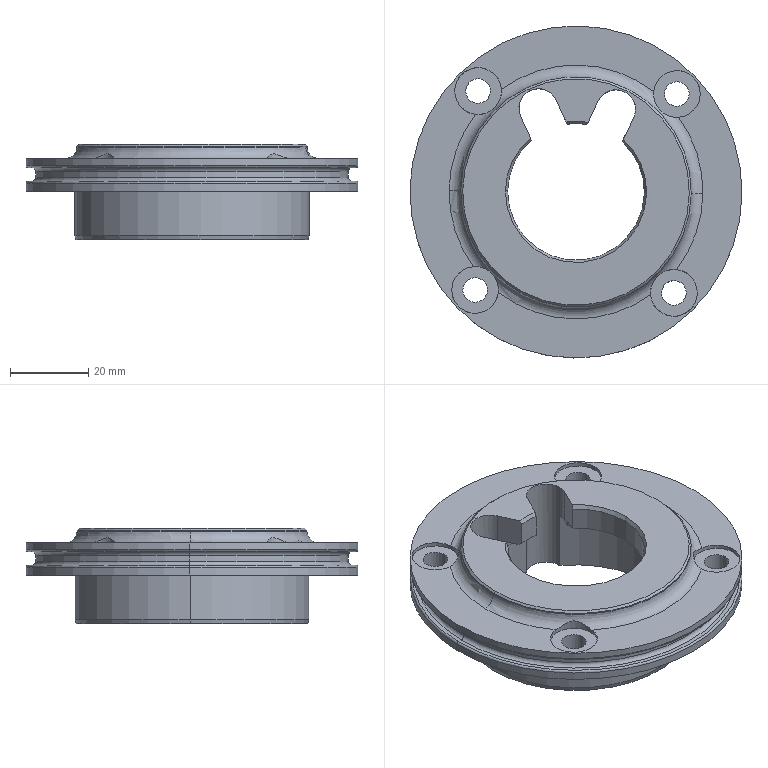Part | SolidWorks | features BaseBody 1 | 1 solid | 81 faces | box 85 x 85 x 24.5 mm | volume 44441 mm3 | cylinder 41 | plane 18 | cone 12 | torus 10 | commonest cylinder face diameters 6.3 x8 12 x8 35 x4 43 x4 52 x4 85 x4